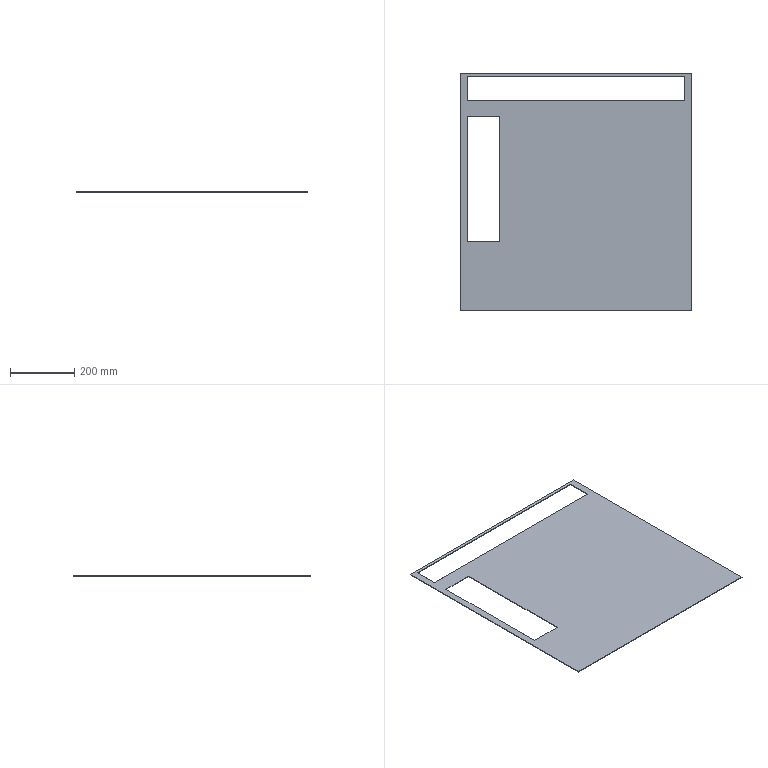Part | STEP file | Guide wheel mechanism revised.sldasm-Part-167 | 1 solid | 14 faces | box 720 x 740 x 2 mm | volume 886350 mm3 | plane 14
STEP:
#1=CARTESIAN_POINT('',(360.,740.,200.));
#2=VERTEX_POINT('',#1);
#3=CARTESIAN_POINT('',(360.,0.,200.));
#4=VERTEX_POINT('',#3);
#5=CARTESIAN_POINT('',(360.,740.,200.));
#6=DIRECTION('',(0.,-1.,0.));
#7=VECTOR('',#6,1000.);
#8=LINE('',#5,#7);
#9=EDGE_CURVE('',#2,#4,#8,.T.);
#10=ORIENTED_EDGE('',*,*,#9,.F.);
#11=CARTESIAN_POINT('',(360.,740.,202.));
#12=VERTEX_POINT('',#11);
#13=CARTESIAN_POINT('',(360.,740.,202.));
#14=DIRECTION('',(0.,0.,-1.));
#15=VECTOR('',#14,1000.);
#16=LINE('',#13,#15);
#17=EDGE_CURVE('',#12,#2,#16,.T.);
#18=ORIENTED_EDGE('',*,*,#17,.F.);
#19=CARTESIAN_POINT('',(360.,0.,202.));
#20=VERTEX_POINT('',#19);
#21=CARTESIAN_POINT('',(360.,740.,202.));
#22=DIRECTION('',(0.,-1.,0.));
#23=VECTOR('',#22,1000.);
#24=LINE('',#21,#23);
#25=EDGE_CURVE('',#12,#20,#24,.T.);
#26=ORIENTED_EDGE('',*,*,#25,.T.);
#27=CARTESIAN_POINT('',(360.,0.,202.));
#28=DIRECTION('',(0.,0.,-1.));
#29=VECTOR('',#28,1000.);
#30=LINE('',#27,#29);
#31=EDGE_CURVE('',#20,#4,#30,.T.);
#32=ORIENTED_EDGE('',*,*,#31,.T.);
#33=EDGE_LOOP('',(#10,#18,#26,#32));
#34=FACE_OUTER_BOUND('',#33,.T.);
#35=CARTESIAN_POINT('',(360.,740.,202.));
#36=DIRECTION('',(1.,0.,0.));
#37=DIRECTION('',(0.,1.,0.));
#38=AXIS2_PLACEMENT_3D('',#35,#36,#37);
#39=PLANE('',#38);
#40=ADVANCED_FACE('',(#34),#39,.T.);
#41=CARTESIAN_POINT('',(-360.,740.,200.));
#42=VERTEX_POINT('',#41);
#43=CARTESIAN_POINT('',(360.,740.,200.));
#44=DIRECTION('',(1.,0.,0.));
#45=VECTOR('',#44,1000.);
#46=LINE('',#43,#45);
#47=EDGE_CURVE('',#42,#2,#46,.T.);
#48=ORIENTED_EDGE('',*,*,#47,.F.);
#49=CARTESIAN_POINT('',(-360.,740.,202.));
#50=VERTEX_POINT('',#49);
#51=CARTESIAN_POINT('',(-360.,740.,202.));
#52=DIRECTION('',(0.,0.,-1.));
#53=VECTOR('',#52,1000.);
#54=LINE('',#51,#53);
#55=EDGE_CURVE('',#50,#42,#54,.T.);
#56=ORIENTED_EDGE('',*,*,#55,.F.);
#57=CARTESIAN_POINT('',(360.,740.,202.));
#58=DIRECTION('',(1.,0.,0.));
#59=VECTOR('',#58,1000.);
#60=LINE('',#57,#59);
#61=EDGE_CURVE('',#50,#12,#60,.T.);
#62=ORIENTED_EDGE('',*,*,#61,.T.);
#63=ORIENTED_EDGE('',*,*,#17,.T.);
#64=EDGE_LOOP('',(#48,#56,#62,#63));
#65=FACE_OUTER_BOUND('',#64,.T.);
#66=CARTESIAN_POINT('',(360.,740.,202.));
#67=DIRECTION('',(0.,1.,0.));
#68=DIRECTION('',(-1.,0.,0.));
#69=AXIS2_PLACEMENT_3D('',#66,#67,#68);
#70=PLANE('',#69);
#71=ADVANCED_FACE('',(#65),#70,.T.);
#72=CARTESIAN_POINT('',(-360.,0.,200.));
#73=VERTEX_POINT('',#72);
#74=CARTESIAN_POINT('',(-360.,740.,200.));
#75=DIRECTION('',(0.,1.,0.));
#76=VECTOR('',#75,1000.);
#77=LINE('',#74,#76);
#78=EDGE_CURVE('',#73,#42,#77,.T.);
#79=ORIENTED_EDGE('',*,*,#78,.F.);
#80=CARTESIAN_POINT('',(-360.,0.,202.));
#81=VERTEX_POINT('',#80);
#82=CARTESIAN_POINT('',(-360.,0.,202.));
#83=DIRECTION('',(0.,0.,-1.));
#84=VECTOR('',#83,1000.);
#85=LINE('',#82,#84);
#86=EDGE_CURVE('',#81,#73,#85,.T.);
#87=ORIENTED_EDGE('',*,*,#86,.F.);
#88=CARTESIAN_POINT('',(-360.,740.,202.));
#89=DIRECTION('',(0.,1.,0.));
#90=VECTOR('',#89,1000.);
#91=LINE('',#88,#90);
#92=EDGE_CURVE('',#81,#50,#91,.T.);
#93=ORIENTED_EDGE('',*,*,#92,.T.);
#94=ORIENTED_EDGE('',*,*,#55,.T.);
#95=EDGE_LOOP('',(#79,#87,#93,#94));
#96=FACE_OUTER_BOUND('',#95,.T.);
#97=CARTESIAN_POINT('',(-360.,740.,202.));
#98=DIRECTION('',(-1.,0.,0.));
#99=DIRECTION('',(0.,-1.,0.));
#100=AXIS2_PLACEMENT_3D('',#97,#98,#99);
#101=PLANE('',#100);
#102=ADVANCED_FACE('',(#96),#101,.T.);
#103=CARTESIAN_POINT('',(360.,0.,200.));
#104=DIRECTION('',(-1.,0.,0.));
#105=VECTOR('',#104,1000.);
#106=LINE('',#103,#105);
#107=EDGE_CURVE('',#4,#73,#106,.T.);
#108=ORIENTED_EDGE('',*,*,#107,.F.);
#109=ORIENTED_EDGE('',*,*,#31,.F.);
#110=CARTESIAN_POINT('',(360.,0.,202.));
#111=DIRECTION('',(-1.,0.,0.));
#112=VECTOR('',#111,1000.);
#113=LINE('',#110,#112);
#114=EDGE_CURVE('',#20,#81,#113,.T.);
#115=ORIENTED_EDGE('',*,*,#114,.T.);
#116=ORIENTED_EDGE('',*,*,#86,.T.);
#117=EDGE_LOOP('',(#108,#109,#115,#116));
#118=FACE_OUTER_BOUND('',#117,.T.);
#119=CARTESIAN_POINT('',(360.,0.,202.));
#120=DIRECTION('',(0.,-1.,0.));
#121=DIRECTION('',(0.,0.,-1.));
#122=AXIS2_PLACEMENT_3D('',#119,#120,#121);
#123=PLANE('',#122);
#124=ADVANCED_FACE('',(#118),#123,.T.);
#125=CARTESIAN_POINT('',(-237.5,215.,202.));
#126=VERTEX_POINT('',#125);
#127=CARTESIAN_POINT('',(-337.5,215.,202.));
#128=VERTEX_POINT('',#127);
#129=CARTESIAN_POINT('',(-337.5,215.,202.));
#130=DIRECTION('',(-1.,0.,0.));
#131=VECTOR('',#130,1000.);
#132=LINE('',#129,#131);
#133=EDGE_CURVE('',#126,#128,#132,.T.);
#134=ORIENTED_EDGE('',*,*,#133,.T.);
#135=CARTESIAN_POINT('',(-337.5,605.,202.));
#136=VERTEX_POINT('',#135);
#137=CARTESIAN_POINT('',(-337.5,605.,202.));
#138=DIRECTION('',(0.,1.,0.));
#139=VECTOR('',#138,1000.);
#140=LINE('',#137,#139);
#141=EDGE_CURVE('',#128,#136,#140,.T.);
#142=ORIENTED_EDGE('',*,*,#141,.T.);
#143=CARTESIAN_POINT('',(-237.5,605.,202.));
#144=VERTEX_POINT('',#143);
#145=CARTESIAN_POINT('',(-337.5,605.,202.));
#146=DIRECTION('',(1.,0.,0.));
#147=VECTOR('',#146,1000.);
#148=LINE('',#145,#147);
#149=EDGE_CURVE('',#136,#144,#148,.T.);
#150=ORIENTED_EDGE('',*,*,#149,.T.);
#151=CARTESIAN_POINT('',(-237.5,605.,202.));
#152=DIRECTION('',(0.,-1.,0.));
#153=VECTOR('',#152,1000.);
#154=LINE('',#151,#153);
#155=EDGE_CURVE('',#144,#126,#154,.T.);
#156=ORIENTED_EDGE('',*,*,#155,.T.);
#157=EDGE_LOOP('',(#134,#142,#150,#156));
#158=FACE_BOUND('',#157,.T.);
#159=CARTESIAN_POINT('',(337.5,655.,202.));
#160=VERTEX_POINT('',#159);
#161=CARTESIAN_POINT('',(-337.5,655.,202.));
#162=VERTEX_POINT('',#161);
#163=CARTESIAN_POINT('',(-337.5,655.,202.));
#164=DIRECTION('',(-1.,0.,0.));
#165=VECTOR('',#164,1000.);
#166=LINE('',#163,#165);
#167=EDGE_CURVE('',#160,#162,#166,.T.);
#168=ORIENTED_EDGE('',*,*,#167,.T.);
#169=CARTESIAN_POINT('',(-337.5,730.,202.));
#170=VERTEX_POINT('',#169);
#171=CARTESIAN_POINT('',(-337.5,730.,202.));
#172=DIRECTION('',(0.,1.,0.));
#173=VECTOR('',#172,1000.);
#174=LINE('',#171,#173);
#175=EDGE_CURVE('',#162,#170,#174,.T.);
#176=ORIENTED_EDGE('',*,*,#175,.T.);
#177=CARTESIAN_POINT('',(337.5,730.,202.));
#178=VERTEX_POINT('',#177);
#179=CARTESIAN_POINT('',(-337.5,730.,202.));
#180=DIRECTION('',(1.,0.,0.));
#181=VECTOR('',#180,1000.);
#182=LINE('',#179,#181);
#183=EDGE_CURVE('',#170,#178,#182,.T.);
#184=ORIENTED_EDGE('',*,*,#183,.T.);
#185=CARTESIAN_POINT('',(337.5,730.,202.));
#186=DIRECTION('',(0.,-1.,0.));
#187=VECTOR('',#186,1000.);
#188=LINE('',#185,#187);
#189=EDGE_CURVE('',#178,#160,#188,.T.);
#190=ORIENTED_EDGE('',*,*,#189,.T.);
#191=EDGE_LOOP('',(#168,#176,#184,#190));
#192=FACE_BOUND('',#191,.T.);
#193=ORIENTED_EDGE('',*,*,#25,.F.);
#194=ORIENTED_EDGE('',*,*,#61,.F.);
#195=ORIENTED_EDGE('',*,*,#92,.F.);
#196=ORIENTED_EDGE('',*,*,#114,.F.);
#197=EDGE_LOOP('',(#193,#194,#195,#196));
#198=FACE_OUTER_BOUND('',#197,.T.);
#199=CARTESIAN_POINT('',(0.,0.,202.));
#200=DIRECTION('',(0.,0.,-1.));
#201=DIRECTION('',(-1.,0.,0.));
#202=AXIS2_PLACEMENT_3D('',#199,#200,#201);
#203=PLANE('',#202);
#204=ADVANCED_FACE('',(#158,#192,#198),#203,.F.);
#205=CARTESIAN_POINT('',(-337.5,215.,200.));
#206=VERTEX_POINT('',#205);
#207=CARTESIAN_POINT('',(-337.5,605.,200.));
#208=VERTEX_POINT('',#207);
#209=CARTESIAN_POINT('',(-337.5,605.,200.));
#210=DIRECTION('',(0.,1.,0.));
#211=VECTOR('',#210,1000.);
#212=LINE('',#209,#211);
#213=EDGE_CURVE('',#206,#208,#212,.T.);
#214=ORIENTED_EDGE('',*,*,#213,.F.);
#215=CARTESIAN_POINT('',(-237.5,215.,200.));
#216=VERTEX_POINT('',#215);
#217=CARTESIAN_POINT('',(-337.5,215.,200.));
#218=DIRECTION('',(-1.,0.,0.));
#219=VECTOR('',#218,1000.);
#220=LINE('',#217,#219);
#221=EDGE_CURVE('',#216,#206,#220,.T.);
#222=ORIENTED_EDGE('',*,*,#221,.F.);
#223=CARTESIAN_POINT('',(-237.5,605.,200.));
#224=VERTEX_POINT('',#223);
#225=CARTESIAN_POINT('',(-237.5,605.,200.));
#226=DIRECTION('',(0.,-1.,0.));
#227=VECTOR('',#226,1000.);
#228=LINE('',#225,#227);
#229=EDGE_CURVE('',#224,#216,#228,.T.);
#230=ORIENTED_EDGE('',*,*,#229,.F.);
#231=CARTESIAN_POINT('',(-337.5,605.,200.));
#232=DIRECTION('',(1.,0.,0.));
#233=VECTOR('',#232,1000.);
#234=LINE('',#231,#233);
#235=EDGE_CURVE('',#208,#224,#234,.T.);
#236=ORIENTED_EDGE('',*,*,#235,.F.);
#237=EDGE_LOOP('',(#214,#222,#230,#236));
#238=FACE_BOUND('',#237,.T.);
#239=CARTESIAN_POINT('',(-337.5,655.,200.));
#240=VERTEX_POINT('',#239);
#241=CARTESIAN_POINT('',(-337.5,730.,200.));
#242=VERTEX_POINT('',#241);
#243=CARTESIAN_POINT('',(-337.5,730.,200.));
#244=DIRECTION('',(0.,1.,0.));
#245=VECTOR('',#244,1000.);
#246=LINE('',#243,#245);
#247=EDGE_CURVE('',#240,#242,#246,.T.);
#248=ORIENTED_EDGE('',*,*,#247,.F.);
#249=CARTESIAN_POINT('',(337.5,655.,200.));
#250=VERTEX_POINT('',#249);
#251=CARTESIAN_POINT('',(-337.5,655.,200.));
#252=DIRECTION('',(-1.,0.,0.));
#253=VECTOR('',#252,1000.);
#254=LINE('',#251,#253);
#255=EDGE_CURVE('',#250,#240,#254,.T.);
#256=ORIENTED_EDGE('',*,*,#255,.F.);
#257=CARTESIAN_POINT('',(337.5,730.,200.));
#258=VERTEX_POINT('',#257);
#259=CARTESIAN_POINT('',(337.5,730.,200.));
#260=DIRECTION('',(0.,-1.,0.));
#261=VECTOR('',#260,1000.);
#262=LINE('',#259,#261);
#263=EDGE_CURVE('',#258,#250,#262,.T.);
#264=ORIENTED_EDGE('',*,*,#263,.F.);
#265=CARTESIAN_POINT('',(-337.5,730.,200.));
#266=DIRECTION('',(1.,0.,0.));
#267=VECTOR('',#266,1000.);
#268=LINE('',#265,#267);
#269=EDGE_CURVE('',#242,#258,#268,.T.);
#270=ORIENTED_EDGE('',*,*,#269,.F.);
#271=EDGE_LOOP('',(#248,#256,#264,#270));
#272=FACE_BOUND('',#271,.T.);
#273=ORIENTED_EDGE('',*,*,#9,.T.);
#274=ORIENTED_EDGE('',*,*,#107,.T.);
#275=ORIENTED_EDGE('',*,*,#78,.T.);
#276=ORIENTED_EDGE('',*,*,#47,.T.);
#277=EDGE_LOOP('',(#273,#274,#275,#276));
#278=FACE_OUTER_BOUND('',#277,.T.);
#279=CARTESIAN_POINT('',(0.,0.,200.));
#280=DIRECTION('',(0.,0.,-1.));
#281=DIRECTION('',(-1.,0.,0.));
#282=AXIS2_PLACEMENT_3D('',#279,#280,#281);
#283=PLANE('',#282);
#284=ADVANCED_FACE('',(#238,#272,#278),#283,.T.);
#285=ORIENTED_EDGE('',*,*,#247,.T.);
#286=CARTESIAN_POINT('',(-337.5,730.,202.));
#287=DIRECTION('',(0.,0.,-1.));
#288=VECTOR('',#287,1000.);
#289=LINE('',#286,#288);
#290=EDGE_CURVE('',#170,#242,#289,.T.);
#291=ORIENTED_EDGE('',*,*,#290,.F.);
#292=ORIENTED_EDGE('',*,*,#175,.F.);
#293=CARTESIAN_POINT('',(-337.5,655.,202.));
#294=DIRECTION('',(0.,0.,-1.));
#295=VECTOR('',#294,1000.);
#296=LINE('',#293,#295);
#297=EDGE_CURVE('',#162,#240,#296,.T.);
#298=ORIENTED_EDGE('',*,*,#297,.T.);
#299=EDGE_LOOP('',(#285,#291,#292,#298));
#300=FACE_OUTER_BOUND('',#299,.T.);
#301=CARTESIAN_POINT('',(-337.5,730.,202.));
#302=DIRECTION('',(-1.,0.,0.));
#303=DIRECTION('',(0.,-1.,0.));
#304=AXIS2_PLACEMENT_3D('',#301,#302,#303);
#305=PLANE('',#304);
#306=ADVANCED_FACE('',(#300),#305,.F.);
#307=ORIENTED_EDGE('',*,*,#255,.T.);
#308=ORIENTED_EDGE('',*,*,#297,.F.);
#309=ORIENTED_EDGE('',*,*,#167,.F.);
#310=CARTESIAN_POINT('',(337.5,655.,202.));
#311=DIRECTION('',(0.,0.,-1.));
#312=VECTOR('',#311,1000.);
#313=LINE('',#310,#312);
#314=EDGE_CURVE('',#160,#250,#313,.T.);
#315=ORIENTED_EDGE('',*,*,#314,.T.);
#316=EDGE_LOOP('',(#307,#308,#309,#315));
#317=FACE_OUTER_BOUND('',#316,.T.);
#318=CARTESIAN_POINT('',(-337.5,655.,202.));
#319=DIRECTION('',(0.,-1.,0.));
#320=DIRECTION('',(1.,0.,0.));
#321=AXIS2_PLACEMENT_3D('',#318,#319,#320);
#322=PLANE('',#321);
#323=ADVANCED_FACE('',(#317),#322,.F.);
#324=ORIENTED_EDGE('',*,*,#263,.T.);
#325=ORIENTED_EDGE('',*,*,#314,.F.);
#326=ORIENTED_EDGE('',*,*,#189,.F.);
#327=CARTESIAN_POINT('',(337.5,730.,202.));
#328=DIRECTION('',(0.,0.,-1.));
#329=VECTOR('',#328,1000.);
#330=LINE('',#327,#329);
#331=EDGE_CURVE('',#178,#258,#330,.T.);
#332=ORIENTED_EDGE('',*,*,#331,.T.);
#333=EDGE_LOOP('',(#324,#325,#326,#332));
#334=FACE_OUTER_BOUND('',#333,.T.);
#335=CARTESIAN_POINT('',(337.5,730.,202.));
#336=DIRECTION('',(1.,0.,0.));
#337=DIRECTION('',(0.,1.,0.));
#338=AXIS2_PLACEMENT_3D('',#335,#336,#337);
#339=PLANE('',#338);
#340=ADVANCED_FACE('',(#334),#339,.F.);
#341=ORIENTED_EDGE('',*,*,#269,.T.);
#342=ORIENTED_EDGE('',*,*,#331,.F.);
#343=ORIENTED_EDGE('',*,*,#183,.F.);
#344=ORIENTED_EDGE('',*,*,#290,.T.);
#345=EDGE_LOOP('',(#341,#342,#343,#344));
#346=FACE_OUTER_BOUND('',#345,.T.);
#347=CARTESIAN_POINT('',(-337.5,730.,202.));
#348=DIRECTION('',(0.,1.,0.));
#349=DIRECTION('',(-1.,0.,0.));
#350=AXIS2_PLACEMENT_3D('',#347,#348,#349);
#351=PLANE('',#350);
#352=ADVANCED_FACE('',(#346),#351,.F.);
#353=ORIENTED_EDGE('',*,*,#213,.T.);
#354=CARTESIAN_POINT('',(-337.5,605.,202.));
#355=DIRECTION('',(0.,0.,-1.));
#356=VECTOR('',#355,1000.);
#357=LINE('',#354,#356);
#358=EDGE_CURVE('',#136,#208,#357,.T.);
#359=ORIENTED_EDGE('',*,*,#358,.F.);
#360=ORIENTED_EDGE('',*,*,#141,.F.);
#361=CARTESIAN_POINT('',(-337.5,215.,202.));
#362=DIRECTION('',(0.,0.,-1.));
#363=VECTOR('',#362,1000.);
#364=LINE('',#361,#363);
#365=EDGE_CURVE('',#128,#206,#364,.T.);
#366=ORIENTED_EDGE('',*,*,#365,.T.);
#367=EDGE_LOOP('',(#353,#359,#360,#366));
#368=FACE_OUTER_BOUND('',#367,.T.);
#369=CARTESIAN_POINT('',(-337.5,605.,202.));
#370=DIRECTION('',(-1.,0.,0.));
#371=DIRECTION('',(0.,-1.,0.));
#372=AXIS2_PLACEMENT_3D('',#369,#370,#371);
#373=PLANE('',#372);
#374=ADVANCED_FACE('',(#368),#373,.F.);
#375=ORIENTED_EDGE('',*,*,#221,.T.);
#376=ORIENTED_EDGE('',*,*,#365,.F.);
#377=ORIENTED_EDGE('',*,*,#133,.F.);
#378=CARTESIAN_POINT('',(-237.5,215.,202.));
#379=DIRECTION('',(0.,0.,-1.));
#380=VECTOR('',#379,1000.);
#381=LINE('',#378,#380);
#382=EDGE_CURVE('',#126,#216,#381,.T.);
#383=ORIENTED_EDGE('',*,*,#382,.T.);
#384=EDGE_LOOP('',(#375,#376,#377,#383));
#385=FACE_OUTER_BOUND('',#384,.T.);
#386=CARTESIAN_POINT('',(-337.5,215.,202.));
#387=DIRECTION('',(0.,-1.,0.));
#388=DIRECTION('',(0.,0.,-1.));
#389=AXIS2_PLACEMENT_3D('',#386,#387,#388);
#390=PLANE('',#389);
#391=ADVANCED_FACE('',(#385),#390,.F.);
#392=ORIENTED_EDGE('',*,*,#229,.T.);
#393=ORIENTED_EDGE('',*,*,#382,.F.);
#394=ORIENTED_EDGE('',*,*,#155,.F.);
#395=CARTESIAN_POINT('',(-237.5,605.,202.));
#396=DIRECTION('',(0.,0.,-1.));
#397=VECTOR('',#396,1000.);
#398=LINE('',#395,#397);
#399=EDGE_CURVE('',#144,#224,#398,.T.);
#400=ORIENTED_EDGE('',*,*,#399,.T.);
#401=EDGE_LOOP('',(#392,#393,#394,#400));
#402=FACE_OUTER_BOUND('',#401,.T.);
#403=CARTESIAN_POINT('',(-237.5,605.,202.));
#404=DIRECTION('',(1.,0.,0.));
#405=DIRECTION('',(0.,1.,0.));
#406=AXIS2_PLACEMENT_3D('',#403,#404,#405);
#407=PLANE('',#406);
#408=ADVANCED_FACE('',(#402),#407,.F.);
#409=ORIENTED_EDGE('',*,*,#235,.T.);
#410=ORIENTED_EDGE('',*,*,#399,.F.);
#411=ORIENTED_EDGE('',*,*,#149,.F.);
#412=ORIENTED_EDGE('',*,*,#358,.T.);
#413=EDGE_LOOP('',(#409,#410,#411,#412));
#414=FACE_OUTER_BOUND('',#413,.T.);
#415=CARTESIAN_POINT('',(-337.5,605.,202.));
#416=DIRECTION('',(0.,1.,0.));
#417=DIRECTION('',(0.,0.,1.));
#418=AXIS2_PLACEMENT_3D('',#415,#416,#417);
#419=PLANE('',#418);
#420=ADVANCED_FACE('',(#414),#419,.F.);
#421=CLOSED_SHELL('',(#40,#71,#102,#124,#204,#284,#306,#323,#340,#352,#374,#391,#408,#420));
#422=MANIFOLD_SOLID_BREP('',#421);
#423=CARTESIAN_POINT('',(0.,0.,0.));
#424=DIRECTION('',(0.,0.,1.));
#425=DIRECTION('',(1.,0.,0.));
#426=AXIS2_PLACEMENT_3D('',#423,#424,#425);
#427=(LENGTH_UNIT()NAMED_UNIT(*)SI_UNIT(.MILLI.,.METRE.));
#428=UNCERTAINTY_MEASURE_WITH_UNIT(LENGTH_MEASURE(0.00001),#427,'','');
#429=(NAMED_UNIT(*)PLANE_ANGLE_UNIT()SI_UNIT($,.RADIAN.));
#430=(NAMED_UNIT(*)SI_UNIT($,.STERADIAN.)SOLID_ANGLE_UNIT());
#431=(GEOMETRIC_REPRESENTATION_CONTEXT(3)GLOBAL_UNCERTAINTY_ASSIGNED_CONTEXT((#428))GLOBAL_UNIT_ASSIGNED_CONTEXT((#427,#429,#430))REPRESENTATION_CONTEXT('',''));
#432=ADVANCED_BREP_SHAPE_REPRESENTATION('',(#422,#426),#431);